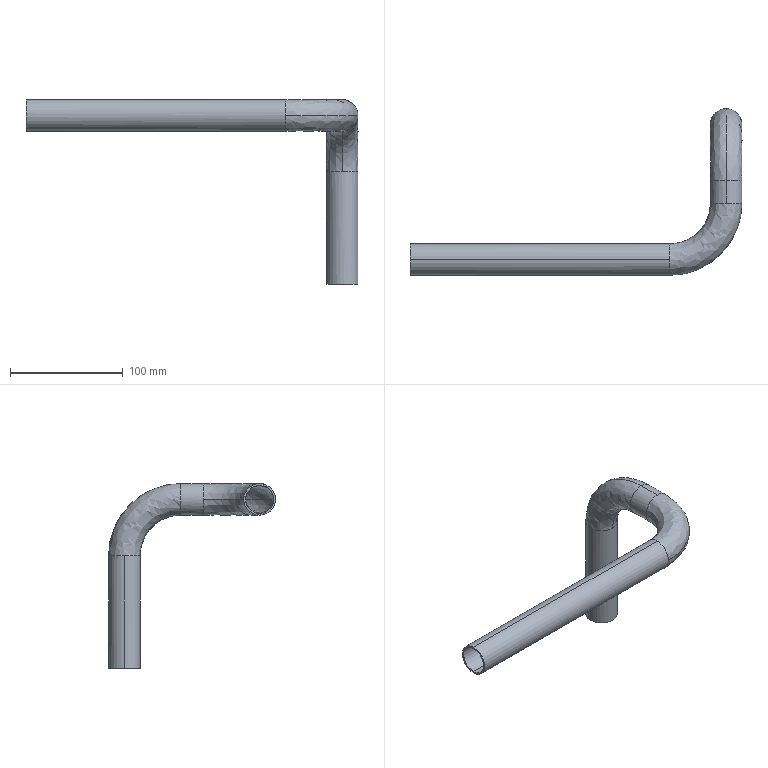Part | STEP file | copper tube 14_default_machined_ | 1 solid | 22 faces | box 294.5 x 148 x 164 mm | volume 63386 mm3 | cylinder 12 | spline 8 | plane 2 | commonest cylinder face diameters 25 x6 28 x6